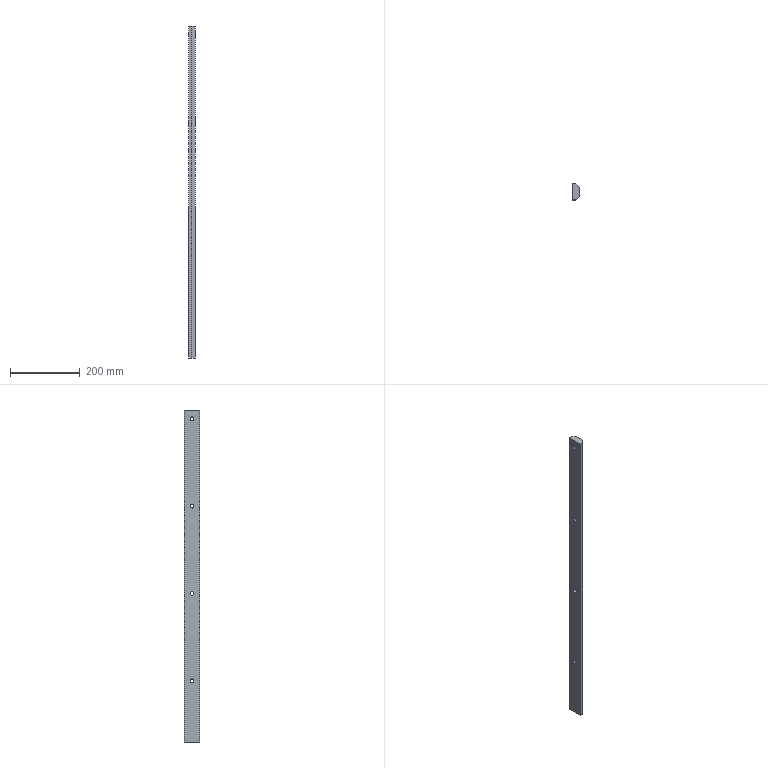Part | STEP file | PN_0053_protective stopper | 1 solid | 28 faces | box 20 x 45 x 950 mm | volume 744681 mm3 | cylinder 16 | plane 12 | commonest cylinder face diameters 11 x8 18 x8